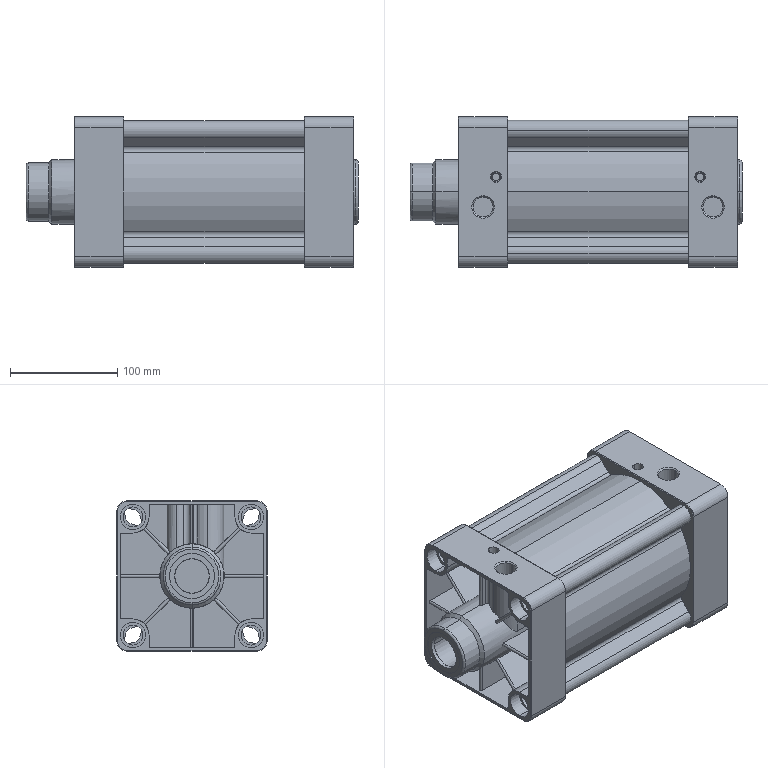Part | STEP file | 1 solid | 393 faces | box 309 x 140 x 140 mm | volume 1499505 mm3 | plane 186 | cylinder 173 | cone 30 | torus 4 | commonest cylinder face diameters 4 x19 3 x18 18.51 x16 23.5 x16 8 x13 6 x12